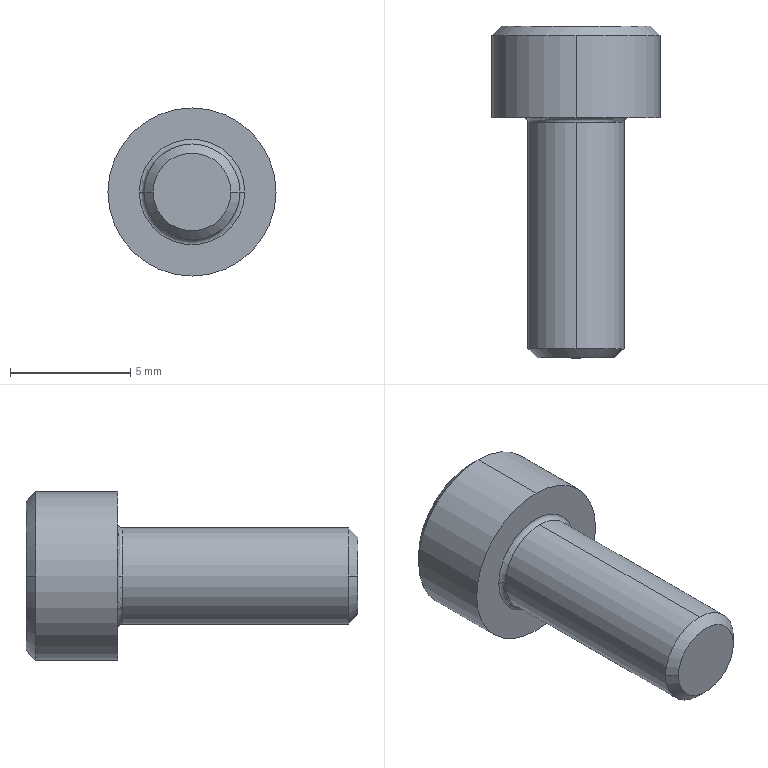Part | NX | 1 solid | 27 faces | box 7 x 13.82 x 7 mm | volume 252.618 mm3 | plane 15 | cone 6 | cylinder 4 | torus 2 | commonest cylinder face diameters 4 x2 7 x2
STEP:
#1=CARTESIAN_POINT('',(8.6,7.32,10.));
#2=VERTEX_POINT('',#1);
#3=CARTESIAN_POINT('',(2.4,7.32,10.));
#4=VERTEX_POINT('',#3);
#5=CARTESIAN_POINT('',(5.5,7.32,10.));
#6=DIRECTION('',(0.,1.,0.));
#7=DIRECTION('',(0.,0.,1.));
#8=AXIS2_PLACEMENT_3D('',#5,#6,#7);
#9=CIRCLE('',#8,3.1);
#10=EDGE_CURVE('',#2,#4,#9,.T.);
#11=ORIENTED_EDGE('',*,*,#10,.F.);
#12=CARTESIAN_POINT('',(9.,6.92,10.));
#13=VERTEX_POINT('',#12);
#14=CARTESIAN_POINT('',(8.8,7.12,10.));
#15=DIRECTION('',(0.7071,-0.7071,0.));
#16=VECTOR('',#15,1000.);
#17=LINE('',#14,#16);
#18=EDGE_CURVE('',#2,#13,#17,.T.);
#19=ORIENTED_EDGE('',*,*,#18,.T.);
#20=CARTESIAN_POINT('',(5.5,6.92,6.5));
#21=VERTEX_POINT('',#20);
#22=CARTESIAN_POINT('',(5.5,6.92,10.));
#23=DIRECTION('',(0.,1.,0.));
#24=DIRECTION('',(0.,0.,1.));
#25=AXIS2_PLACEMENT_3D('',#22,#23,#24);
#26=CIRCLE('',#25,3.5);
#27=EDGE_CURVE('',#13,#21,#26,.T.);
#28=ORIENTED_EDGE('',*,*,#27,.T.);
#29=CARTESIAN_POINT('',(2.,6.92,10.));
#30=VERTEX_POINT('',#29);
#31=CARTESIAN_POINT('',(5.5,6.92,10.));
#32=DIRECTION('',(0.,1.,0.));
#33=DIRECTION('',(0.,0.,1.));
#34=AXIS2_PLACEMENT_3D('',#31,#32,#33);
#35=CIRCLE('',#34,3.5);
#36=EDGE_CURVE('',#21,#30,#35,.T.);
#37=ORIENTED_EDGE('',*,*,#36,.T.);
#38=CARTESIAN_POINT('',(2.2,7.12,10.));
#39=DIRECTION('',(-0.7071,-0.7071,0.));
#40=VECTOR('',#39,1000.);
#41=LINE('',#38,#40);
#42=EDGE_CURVE('',#4,#30,#41,.T.);
#43=ORIENTED_EDGE('',*,*,#42,.F.);
#44=EDGE_LOOP('',(#11,#19,#28,#37,#43));
#45=FACE_BOUND('',#44,.T.);
#46=CARTESIAN_POINT('',(5.5,7.12,10.));
#47=DIRECTION('',(0.,-1.,0.));
#48=DIRECTION('',(-1.,0.,0.));
#49=AXIS2_PLACEMENT_3D('',#46,#47,#48);
#50=CONICAL_SURFACE('',#49,3.3,0.7854);
#51=ADVANCED_FACE('',(#45),#50,.T.);
#52=CARTESIAN_POINT('',(5.5,6.92,13.5));
#53=VERTEX_POINT('',#52);
#54=CARTESIAN_POINT('',(5.5,6.92,10.));
#55=DIRECTION('',(0.,1.,0.));
#56=DIRECTION('',(0.,0.,1.));
#57=AXIS2_PLACEMENT_3D('',#54,#55,#56);
#58=CIRCLE('',#57,3.5);
#59=EDGE_CURVE('',#30,#53,#58,.T.);
#60=ORIENTED_EDGE('',*,*,#59,.F.);
#61=ORIENTED_EDGE('',*,*,#36,.F.);
#62=CARTESIAN_POINT('',(5.5,3.5,6.5));
#63=VERTEX_POINT('',#62);
#64=CARTESIAN_POINT('',(5.5,5.21,6.5));
#65=DIRECTION('',(0.,-1.,0.));
#66=VECTOR('',#65,1000.);
#67=LINE('',#64,#66);
#68=EDGE_CURVE('',#21,#63,#67,.T.);
#69=ORIENTED_EDGE('',*,*,#68,.T.);
#70=CARTESIAN_POINT('',(5.5,3.5,13.5));
#71=VERTEX_POINT('',#70);
#72=CARTESIAN_POINT('',(5.5,3.5,10.));
#73=DIRECTION('',(0.,1.,0.));
#74=DIRECTION('',(0.,0.,1.));
#75=AXIS2_PLACEMENT_3D('',#72,#73,#74);
#76=CIRCLE('',#75,3.5);
#77=EDGE_CURVE('',#63,#71,#76,.T.);
#78=ORIENTED_EDGE('',*,*,#77,.T.);
#79=CARTESIAN_POINT('',(5.5,5.21,13.5));
#80=DIRECTION('',(0.,-1.,0.));
#81=VECTOR('',#80,1000.);
#82=LINE('',#79,#81);
#83=EDGE_CURVE('',#53,#71,#82,.T.);
#84=ORIENTED_EDGE('',*,*,#83,.F.);
#85=EDGE_LOOP('',(#60,#61,#69,#78,#84));
#86=FACE_BOUND('',#85,.T.);
#87=CARTESIAN_POINT('',(5.5,5.21,10.));
#88=DIRECTION('',(0.,-1.,0.));
#89=DIRECTION('',(0.,0.,1.));
#90=AXIS2_PLACEMENT_3D('',#87,#88,#89);
#91=CYLINDRICAL_SURFACE('',#90,3.5);
#92=ADVANCED_FACE('',(#86),#91,.T.);
#93=CARTESIAN_POINT('',(3.3,3.5,10.));
#94=VERTEX_POINT('',#93);
#95=CARTESIAN_POINT('',(7.7,3.5,10.));
#96=VERTEX_POINT('',#95);
#97=CARTESIAN_POINT('',(5.5,3.5,10.));
#98=DIRECTION('',(0.,1.,0.));
#99=DIRECTION('',(0.,0.,1.));
#100=AXIS2_PLACEMENT_3D('',#97,#98,#99);
#101=CIRCLE('',#100,2.2);
#102=EDGE_CURVE('',#94,#96,#101,.T.);
#103=ORIENTED_EDGE('',*,*,#102,.F.);
#104=CARTESIAN_POINT('',(3.5,3.3,10.));
#105=VERTEX_POINT('',#104);
#106=CARTESIAN_POINT('',(3.3,3.3,10.));
#107=DIRECTION('',(0.,0.,1.));
#108=DIRECTION('',(1.,0.,0.));
#109=AXIS2_PLACEMENT_3D('',#106,#107,#108);
#110=CIRCLE('',#109,0.2);
#111=EDGE_CURVE('',#94,#105,#110,.F.);
#112=ORIENTED_EDGE('',*,*,#111,.T.);
#113=CARTESIAN_POINT('',(5.5,3.3,12.));
#114=VERTEX_POINT('',#113);
#115=CARTESIAN_POINT('',(5.5,3.3,10.));
#116=DIRECTION('',(0.,1.,0.));
#117=DIRECTION('',(1.,0.,0.));
#118=AXIS2_PLACEMENT_3D('',#115,#116,#117);
#119=CIRCLE('',#118,2.);
#120=EDGE_CURVE('',#105,#114,#119,.T.);
#121=ORIENTED_EDGE('',*,*,#120,.T.);
#122=CARTESIAN_POINT('',(7.5,3.3,10.));
#123=VERTEX_POINT('',#122);
#124=CARTESIAN_POINT('',(5.5,3.3,10.));
#125=DIRECTION('',(0.,1.,0.));
#126=DIRECTION('',(1.,0.,0.));
#127=AXIS2_PLACEMENT_3D('',#124,#125,#126);
#128=CIRCLE('',#127,2.);
#129=EDGE_CURVE('',#114,#123,#128,.T.);
#130=ORIENTED_EDGE('',*,*,#129,.T.);
#131=CARTESIAN_POINT('',(7.7,3.3,10.));
#132=DIRECTION('',(0.,0.,-1.));
#133=DIRECTION('',(-1.,0.,0.));
#134=AXIS2_PLACEMENT_3D('',#131,#132,#133);
#135=CIRCLE('',#134,0.2);
#136=EDGE_CURVE('',#96,#123,#135,.F.);
#137=ORIENTED_EDGE('',*,*,#136,.F.);
#138=EDGE_LOOP('',(#103,#112,#121,#130,#137));
#139=FACE_BOUND('',#138,.T.);
#140=CARTESIAN_POINT('',(5.5,3.3,10.));
#141=DIRECTION('',(0.,1.,0.));
#142=DIRECTION('',(1.,0.,0.));
#143=AXIS2_PLACEMENT_3D('',#140,#141,#142);
#144=TOROIDAL_SURFACE('',#143,2.2,0.2);
#145=ADVANCED_FACE('',(#139),#144,.F.);
#146=CARTESIAN_POINT('',(5.5,-6.121,8.));
#147=VERTEX_POINT('',#146);
#148=CARTESIAN_POINT('',(3.5,-6.121,10.));
#149=VERTEX_POINT('',#148);
#150=CARTESIAN_POINT('',(5.5,-6.121,10.));
#151=DIRECTION('',(0.,1.,0.));
#152=DIRECTION('',(0.,0.,1.));
#153=AXIS2_PLACEMENT_3D('',#150,#151,#152);
#154=CIRCLE('',#153,2.);
#155=EDGE_CURVE('',#147,#149,#154,.T.);
#156=ORIENTED_EDGE('',*,*,#155,.T.);
#157=CARTESIAN_POINT('',(5.5,-6.121,12.));
#158=VERTEX_POINT('',#157);
#159=CARTESIAN_POINT('',(5.5,-6.121,10.));
#160=DIRECTION('',(0.,1.,0.));
#161=DIRECTION('',(0.,0.,1.));
#162=AXIS2_PLACEMENT_3D('',#159,#160,#161);
#163=CIRCLE('',#162,2.);
#164=EDGE_CURVE('',#149,#158,#163,.T.);
#165=ORIENTED_EDGE('',*,*,#164,.T.);
#166=CARTESIAN_POINT('',(5.5,-1.411,12.));
#167=DIRECTION('',(0.,-1.,0.));
#168=VECTOR('',#167,1000.);
#169=LINE('',#166,#168);
#170=EDGE_CURVE('',#114,#158,#169,.T.);
#171=ORIENTED_EDGE('',*,*,#170,.F.);
#172=ORIENTED_EDGE('',*,*,#120,.F.);
#173=CARTESIAN_POINT('',(5.5,3.3,8.));
#174=VERTEX_POINT('',#173);
#175=CARTESIAN_POINT('',(5.5,3.3,10.));
#176=DIRECTION('',(0.,1.,0.));
#177=DIRECTION('',(1.,0.,0.));
#178=AXIS2_PLACEMENT_3D('',#175,#176,#177);
#179=CIRCLE('',#178,2.);
#180=EDGE_CURVE('',#174,#105,#179,.T.);
#181=ORIENTED_EDGE('',*,*,#180,.F.);
#182=CARTESIAN_POINT('',(5.5,-1.411,8.));
#183=DIRECTION('',(0.,-1.,0.));
#184=VECTOR('',#183,1000.);
#185=LINE('',#182,#184);
#186=EDGE_CURVE('',#174,#147,#185,.T.);
#187=ORIENTED_EDGE('',*,*,#186,.T.);
#188=EDGE_LOOP('',(#156,#165,#171,#172,#181,#187));
#189=FACE_BOUND('',#188,.T.);
#190=CARTESIAN_POINT('',(5.5,-1.411,10.));
#191=DIRECTION('',(0.,-1.,0.));
#192=DIRECTION('',(0.,0.,1.));
#193=AXIS2_PLACEMENT_3D('',#190,#191,#192);
#194=CYLINDRICAL_SURFACE('',#193,2.);
#195=ADVANCED_FACE('',(#189),#194,.T.);
#196=ORIENTED_EDGE('',*,*,#155,.F.);
#197=CARTESIAN_POINT('',(7.5,-6.121,10.));
#198=VERTEX_POINT('',#197);
#199=CARTESIAN_POINT('',(5.5,-6.121,10.));
#200=DIRECTION('',(0.,1.,0.));
#201=DIRECTION('',(0.,0.,1.));
#202=AXIS2_PLACEMENT_3D('',#199,#200,#201);
#203=CIRCLE('',#202,2.);
#204=EDGE_CURVE('',#198,#147,#203,.T.);
#205=ORIENTED_EDGE('',*,*,#204,.F.);
#206=CARTESIAN_POINT('',(7.121,-6.5,10.));
#207=VERTEX_POINT('',#206);
#208=CARTESIAN_POINT('',(7.311,-6.311,10.));
#209=DIRECTION('',(0.7071,0.7071,0.));
#210=VECTOR('',#209,1000.);
#211=LINE('',#208,#210);
#212=EDGE_CURVE('',#207,#198,#211,.T.);
#213=ORIENTED_EDGE('',*,*,#212,.F.);
#214=CARTESIAN_POINT('',(3.879,-6.5,10.));
#215=VERTEX_POINT('',#214);
#216=CARTESIAN_POINT('',(5.5,-6.5,10.));
#217=DIRECTION('',(0.,1.,0.));
#218=DIRECTION('',(0.,0.,1.));
#219=AXIS2_PLACEMENT_3D('',#216,#217,#218);
#220=CIRCLE('',#219,1.621);
#221=EDGE_CURVE('',#207,#215,#220,.T.);
#222=ORIENTED_EDGE('',*,*,#221,.T.);
#223=CARTESIAN_POINT('',(3.689,-6.311,10.));
#224=DIRECTION('',(-0.7071,0.7071,0.));
#225=VECTOR('',#224,1000.);
#226=LINE('',#223,#225);
#227=EDGE_CURVE('',#215,#149,#226,.T.);
#228=ORIENTED_EDGE('',*,*,#227,.T.);
#229=EDGE_LOOP('',(#196,#205,#213,#222,#228));
#230=FACE_BOUND('',#229,.T.);
#231=CARTESIAN_POINT('',(5.5,-6.311,10.));
#232=DIRECTION('',(0.,1.,0.));
#233=DIRECTION('',(1.,0.,0.));
#234=AXIS2_PLACEMENT_3D('',#231,#232,#233);
#235=CONICAL_SURFACE('',#234,1.81,0.7854);
#236=ADVANCED_FACE('',(#230),#235,.T.);
#237=CARTESIAN_POINT('',(4.,5.32,10.));
#238=VERTEX_POINT('',#237);
#239=CARTESIAN_POINT('',(5.5,4.454,10.));
#240=VERTEX_POINT('',#239);
#241=CARTESIAN_POINT('',(4.75,4.887,10.));
#242=DIRECTION('',(-0.866,0.5,0.));
#243=VECTOR('',#242,1000.);
#244=LINE('',#241,#243);
#245=EDGE_CURVE('',#238,#240,#244,.F.);
#246=ORIENTED_EDGE('',*,*,#245,.F.);
#247=CARTESIAN_POINT('',(4.75,5.32,11.299));
#248=VERTEX_POINT('',#247);
#249=CARTESIAN_POINT('',(5.5,5.32,10.));
#250=DIRECTION('',(0.,-1.,0.));
#251=DIRECTION('',(0.,0.,1.));
#252=AXIS2_PLACEMENT_3D('',#249,#250,#251);
#253=CIRCLE('',#252,1.5);
#254=EDGE_CURVE('',#248,#238,#253,.T.);
#255=ORIENTED_EDGE('',*,*,#254,.F.);
#256=CARTESIAN_POINT('',(6.25,5.32,11.299));
#257=VERTEX_POINT('',#256);
#258=CARTESIAN_POINT('',(5.5,5.32,10.));
#259=DIRECTION('',(0.,-1.,0.));
#260=DIRECTION('',(0.,0.,1.));
#261=AXIS2_PLACEMENT_3D('',#258,#259,#260);
#262=CIRCLE('',#261,1.5);
#263=EDGE_CURVE('',#257,#248,#262,.T.);
#264=ORIENTED_EDGE('',*,*,#263,.F.);
#265=CARTESIAN_POINT('',(7.,5.32,10.));
#266=VERTEX_POINT('',#265);
#267=CARTESIAN_POINT('',(5.5,5.32,10.));
#268=DIRECTION('',(0.,-1.,0.));
#269=DIRECTION('',(0.,0.,1.));
#270=AXIS2_PLACEMENT_3D('',#267,#268,#269);
#271=CIRCLE('',#270,1.5);
#272=EDGE_CURVE('',#266,#257,#271,.T.);
#273=ORIENTED_EDGE('',*,*,#272,.F.);
#274=CARTESIAN_POINT('',(6.25,4.887,10.));
#275=DIRECTION('',(0.866,0.5,0.));
#276=VECTOR('',#275,1000.);
#277=LINE('',#274,#276);
#278=EDGE_CURVE('',#266,#240,#277,.F.);
#279=ORIENTED_EDGE('',*,*,#278,.T.);
#280=EDGE_LOOP('',(#246,#255,#264,#273,#279));
#281=FACE_BOUND('',#280,.T.);
#282=CARTESIAN_POINT('',(5.5,4.887,10.));
#283=DIRECTION('',(0.,1.,0.));
#284=DIRECTION('',(1.,0.,0.));
#285=AXIS2_PLACEMENT_3D('',#282,#283,#284);
#286=CONICAL_SURFACE('',#285,0.75,1.047);
#287=ADVANCED_FACE('',(#281),#286,.F.);
#288=ORIENTED_EDGE('',*,*,#10,.T.);
#289=CARTESIAN_POINT('',(5.5,7.32,10.));
#290=DIRECTION('',(0.,1.,0.));
#291=DIRECTION('',(0.,0.,1.));
#292=AXIS2_PLACEMENT_3D('',#289,#290,#291);
#293=CIRCLE('',#292,3.1);
#294=EDGE_CURVE('',#4,#2,#293,.T.);
#295=ORIENTED_EDGE('',*,*,#294,.T.);
#296=EDGE_LOOP('',(#288,#295));
#297=FACE_BOUND('',#296,.T.);
#298=CARTESIAN_POINT('',(5.5,7.32,11.732));
#299=VERTEX_POINT('',#298);
#300=CARTESIAN_POINT('',(4.,7.32,10.866));
#301=VERTEX_POINT('',#300);
#302=CARTESIAN_POINT('',(4.711,7.32,11.276));
#303=DIRECTION('',(-0.866,0.,-0.5));
#304=VECTOR('',#303,1000.);
#305=LINE('',#302,#304);
#306=EDGE_CURVE('',#299,#301,#305,.T.);
#307=ORIENTED_EDGE('',*,*,#306,.T.);
#308=CARTESIAN_POINT('',(4.,7.32,9.134));
#309=VERTEX_POINT('',#308);
#310=CARTESIAN_POINT('',(4.,7.32,10.342));
#311=DIRECTION('',(0.,0.,-1.));
#312=VECTOR('',#311,1000.);
#313=LINE('',#310,#312);
#314=EDGE_CURVE('',#301,#309,#313,.T.);
#315=ORIENTED_EDGE('',*,*,#314,.T.);
#316=CARTESIAN_POINT('',(5.5,7.32,8.268));
#317=VERTEX_POINT('',#316);
#318=CARTESIAN_POINT('',(4.789,7.32,8.678));
#319=DIRECTION('',(0.866,0.,-0.5));
#320=VECTOR('',#319,1000.);
#321=LINE('',#318,#320);
#322=EDGE_CURVE('',#309,#317,#321,.T.);
#323=ORIENTED_EDGE('',*,*,#322,.T.);
#324=CARTESIAN_POINT('',(7.,7.32,9.134));
#325=VERTEX_POINT('',#324);
#326=CARTESIAN_POINT('',(6.961,7.32,9.111));
#327=DIRECTION('',(0.866,0.,0.5));
#328=VECTOR('',#327,1000.);
#329=LINE('',#326,#328);
#330=EDGE_CURVE('',#317,#325,#329,.T.);
#331=ORIENTED_EDGE('',*,*,#330,.T.);
#332=CARTESIAN_POINT('',(7.,7.32,10.866));
#333=VERTEX_POINT('',#332);
#334=CARTESIAN_POINT('',(7.,7.32,11.208));
#335=DIRECTION('',(0.,0.,1.));
#336=VECTOR('',#335,1000.);
#337=LINE('',#334,#336);
#338=EDGE_CURVE('',#325,#333,#337,.T.);
#339=ORIENTED_EDGE('',*,*,#338,.T.);
#340=CARTESIAN_POINT('',(5.539,7.32,11.709));
#341=DIRECTION('',(-0.866,0.,0.5));
#342=VECTOR('',#341,1000.);
#343=LINE('',#340,#342);
#344=EDGE_CURVE('',#333,#299,#343,.T.);
#345=ORIENTED_EDGE('',*,*,#344,.T.);
#346=EDGE_LOOP('',(#307,#315,#323,#331,#339,#345));
#347=FACE_BOUND('',#346,.T.);
#348=CARTESIAN_POINT('',(5.5,7.32,11.55));
#349=DIRECTION('',(0.,1.,0.));
#350=DIRECTION('',(1.,0.,0.));
#351=AXIS2_PLACEMENT_3D('',#348,#349,#350);
#352=PLANE('',#351);
#353=ADVANCED_FACE('',(#297,#347),#352,.T.);
#354=CARTESIAN_POINT('',(6.25,5.32,8.701));
#355=VERTEX_POINT('',#354);
#356=CARTESIAN_POINT('',(5.5,5.32,10.));
#357=DIRECTION('',(0.,-1.,0.));
#358=DIRECTION('',(0.,0.,1.));
#359=AXIS2_PLACEMENT_3D('',#356,#357,#358);
#360=CIRCLE('',#359,1.5);
#361=EDGE_CURVE('',#355,#266,#360,.T.);
#362=ORIENTED_EDGE('',*,*,#361,.T.);
#363=CARTESIAN_POINT('',(7.,5.32,9.134));
#364=VERTEX_POINT('',#363);
#365=CARTESIAN_POINT('',(7.,5.32,9.134));
#366=DIRECTION('',(0.,0.,-1.));
#367=VECTOR('',#366,1000.);
#368=LINE('',#365,#367);
#369=EDGE_CURVE('',#266,#364,#368,.T.);
#370=ORIENTED_EDGE('',*,*,#369,.T.);
#371=CARTESIAN_POINT('',(5.5,5.32,8.268));
#372=DIRECTION('',(-0.866,0.,-0.5));
#373=VECTOR('',#372,1000.);
#374=LINE('',#371,#373);
#375=EDGE_CURVE('',#364,#355,#374,.T.);
#376=ORIENTED_EDGE('',*,*,#375,.T.);
#377=EDGE_LOOP('',(#362,#370,#376));
#378=FACE_BOUND('',#377,.T.);
#379=CARTESIAN_POINT('',(5.5,5.32,10.));
#380=DIRECTION('',(0.,-1.,0.));
#381=DIRECTION('',(0.,0.,-1.));
#382=AXIS2_PLACEMENT_3D('',#379,#380,#381);
#383=PLANE('',#382);
#384=ADVANCED_FACE('',(#378),#383,.F.);
#385=ORIENTED_EDGE('',*,*,#272,.T.);
#386=CARTESIAN_POINT('',(7.,5.32,10.866));
#387=VERTEX_POINT('',#386);
#388=CARTESIAN_POINT('',(7.,5.32,10.866));
#389=DIRECTION('',(0.866,0.,-0.5));
#390=VECTOR('',#389,1000.);
#391=LINE('',#388,#390);
#392=EDGE_CURVE('',#257,#387,#391,.T.);
#393=ORIENTED_EDGE('',*,*,#392,.T.);
#394=CARTESIAN_POINT('',(7.,5.32,9.134));
#395=DIRECTION('',(0.,0.,-1.));
#396=VECTOR('',#395,1000.);
#397=LINE('',#394,#396);
#398=EDGE_CURVE('',#387,#266,#397,.T.);
#399=ORIENTED_EDGE('',*,*,#398,.T.);
#400=EDGE_LOOP('',(#385,#393,#399));
#401=FACE_BOUND('',#400,.T.);
#402=CARTESIAN_POINT('',(5.5,5.32,10.));
#403=DIRECTION('',(0.,-1.,0.));
#404=DIRECTION('',(0.,0.,-1.));
#405=AXIS2_PLACEMENT_3D('',#402,#403,#404);
#406=PLANE('',#405);
#407=ADVANCED_FACE('',(#401),#406,.F.);
#408=ORIENTED_EDGE('',*,*,#263,.T.);
#409=CARTESIAN_POINT('',(5.5,5.32,11.732));
#410=VERTEX_POINT('',#409);
#411=CARTESIAN_POINT('',(5.5,5.32,11.732));
#412=DIRECTION('',(0.866,0.,0.5));
#413=VECTOR('',#412,1000.);
#414=LINE('',#411,#413);
#415=EDGE_CURVE('',#248,#410,#414,.T.);
#416=ORIENTED_EDGE('',*,*,#415,.T.);
#417=CARTESIAN_POINT('',(7.,5.32,10.866));
#418=DIRECTION('',(0.866,0.,-0.5));
#419=VECTOR('',#418,1000.);
#420=LINE('',#417,#419);
#421=EDGE_CURVE('',#410,#257,#420,.T.);
#422=ORIENTED_EDGE('',*,*,#421,.T.);
#423=EDGE_LOOP('',(#408,#416,#422));
#424=FACE_BOUND('',#423,.T.);
#425=CARTESIAN_POINT('',(5.5,5.32,10.));
#426=DIRECTION('',(0.,-1.,0.));
#427=DIRECTION('',(0.,0.,-1.));
#428=AXIS2_PLACEMENT_3D('',#425,#426,#427);
#429=PLANE('',#428);
#430=ADVANCED_FACE('',(#424),#429,.F.);
#431=ORIENTED_EDGE('',*,*,#254,.T.);
#432=CARTESIAN_POINT('',(4.,5.32,10.866));
#433=VERTEX_POINT('',#432);
#434=CARTESIAN_POINT('',(4.,5.32,10.866));
#435=DIRECTION('',(0.,0.,1.));
#436=VECTOR('',#435,1000.);
#437=LINE('',#434,#436);
#438=EDGE_CURVE('',#238,#433,#437,.T.);
#439=ORIENTED_EDGE('',*,*,#438,.T.);
#440=CARTESIAN_POINT('',(5.5,5.32,11.732));
#441=DIRECTION('',(0.866,0.,0.5));
#442=VECTOR('',#441,1000.);
#443=LINE('',#440,#442);
#444=EDGE_CURVE('',#433,#248,#443,.T.);
#445=ORIENTED_EDGE('',*,*,#444,.T.);
#446=EDGE_LOOP('',(#431,#439,#445));
#447=FACE_BOUND('',#446,.T.);
#448=CARTESIAN_POINT('',(5.5,5.32,10.));
#449=DIRECTION('',(0.,-1.,0.));
#450=DIRECTION('',(0.,0.,-1.));
#451=AXIS2_PLACEMENT_3D('',#448,#449,#450);
#452=PLANE('',#451);
#453=ADVANCED_FACE('',(#447),#452,.F.);
#454=CARTESIAN_POINT('',(4.75,5.32,8.701));
#455=VERTEX_POINT('',#454);
#456=CARTESIAN_POINT('',(5.5,5.32,10.));
#457=DIRECTION('',(0.,-1.,0.));
#458=DIRECTION('',(0.,0.,1.));
#459=AXIS2_PLACEMENT_3D('',#456,#457,#458);
#460=CIRCLE('',#459,1.5);
#461=EDGE_CURVE('',#238,#455,#460,.T.);
#462=ORIENTED_EDGE('',*,*,#461,.T.);
#463=CARTESIAN_POINT('',(4.,5.32,9.134));
#464=VERTEX_POINT('',#463);
#465=CARTESIAN_POINT('',(4.,5.32,9.134));
#466=DIRECTION('',(-0.866,0.,0.5));
#467=VECTOR('',#466,1000.);
#468=LINE('',#465,#467);
#469=EDGE_CURVE('',#455,#464,#468,.T.);
#470=ORIENTED_EDGE('',*,*,#469,.T.);
#471=CARTESIAN_POINT('',(4.,5.32,10.866));
#472=DIRECTION('',(0.,0.,1.));
#473=VECTOR('',#472,1000.);
#474=LINE('',#471,#473);
#475=EDGE_CURVE('',#464,#238,#474,.T.);
#476=ORIENTED_EDGE('',*,*,#475,.T.);
#477=EDGE_LOOP('',(#462,#470,#476));
#478=FACE_BOUND('',#477,.T.);
#479=CARTESIAN_POINT('',(5.5,5.32,10.));
#480=DIRECTION('',(0.,-1.,0.));
#481=DIRECTION('',(0.,0.,-1.));
#482=AXIS2_PLACEMENT_3D('',#479,#480,#481);
#483=PLANE('',#482);
#484=ADVANCED_FACE('',(#478),#483,.F.);
#485=CARTESIAN_POINT('',(5.5,5.32,10.));
#486=DIRECTION('',(0.,-1.,0.));
#487=DIRECTION('',(0.,0.,1.));
#488=AXIS2_PLACEMENT_3D('',#485,#486,#487);
#489=CIRCLE('',#488,1.5);
#490=EDGE_CURVE('',#455,#355,#489,.T.);
#491=ORIENTED_EDGE('',*,*,#490,.T.);
#492=CARTESIAN_POINT('',(5.5,5.32,8.268));
#493=VERTEX_POINT('',#492);
#494=CARTESIAN_POINT('',(5.5,5.32,8.268));
#495=DIRECTION('',(-0.866,0.,-0.5));
#496=VECTOR('',#495,1000.);
#497=LINE('',#494,#496);
#498=EDGE_CURVE('',#355,#493,#497,.T.);
#499=ORIENTED_EDGE('',*,*,#498,.T.);
#500=CARTESIAN_POINT('',(4.,5.32,9.134));
#501=DIRECTION('',(-0.866,0.,0.5));
#502=VECTOR('',#501,1000.);
#503=LINE('',#500,#502);
#504=EDGE_CURVE('',#493,#455,#503,.T.);
#505=ORIENTED_EDGE('',*,*,#504,.T.);
#506=EDGE_LOOP('',(#491,#499,#505));
#507=FACE_BOUND('',#506,.T.);
#508=CARTESIAN_POINT('',(5.5,5.32,10.));
#509=DIRECTION('',(0.,-1.,0.));
#510=DIRECTION('',(0.,0.,-1.));
#511=AXIS2_PLACEMENT_3D('',#508,#509,#510);
#512=PLANE('',#511);
#513=ADVANCED_FACE('',(#507),#512,.F.);
#514=ORIENTED_EDGE('',*,*,#444,.F.);
#515=CARTESIAN_POINT('',(4.,7.32,10.866));
#516=DIRECTION('',(0.,-1.,0.));
#517=VECTOR('',#516,1000.);
#518=LINE('',#515,#517);
#519=EDGE_CURVE('',#301,#433,#518,.T.);
#520=ORIENTED_EDGE('',*,*,#519,.F.);
#521=ORIENTED_EDGE('',*,*,#306,.F.);
#522=CARTESIAN_POINT('',(5.5,7.32,11.732));
#523=DIRECTION('',(0.,-1.,0.));
#524=VECTOR('',#523,1000.);
#525=LINE('',#522,#524);
#526=EDGE_CURVE('',#299,#410,#525,.T.);
#527=ORIENTED_EDGE('',*,*,#526,.T.);
#528=ORIENTED_EDGE('',*,*,#415,.F.);
#529=EDGE_LOOP('',(#514,#520,#521,#527,#528));
#530=FACE_BOUND('',#529,.T.);
#531=CARTESIAN_POINT('',(4.,7.32,10.866));
#532=DIRECTION('',(-0.5,0.,0.866));
#533=DIRECTION('',(0.,1.,0.));
#534=AXIS2_PLACEMENT_3D('',#531,#532,#533);
#535=PLANE('',#534);
#536=ADVANCED_FACE('',(#530),#535,.F.);
#537=ORIENTED_EDGE('',*,*,#421,.F.);
#538=ORIENTED_EDGE('',*,*,#526,.F.);
#539=ORIENTED_EDGE('',*,*,#344,.F.);
#540=CARTESIAN_POINT('',(7.,7.32,10.866));
#541=DIRECTION('',(0.,-1.,0.));
#542=VECTOR('',#541,1000.);
#543=LINE('',#540,#542);
#544=EDGE_CURVE('',#333,#387,#543,.T.);
#545=ORIENTED_EDGE('',*,*,#544,.T.);
#546=ORIENTED_EDGE('',*,*,#392,.F.);
#547=EDGE_LOOP('',(#537,#538,#539,#545,#546));
#548=FACE_BOUND('',#547,.T.);
#549=CARTESIAN_POINT('',(5.5,7.32,11.732));
#550=DIRECTION('',(0.5,0.,0.866));
#551=DIRECTION('',(0.,-1.,0.));
#552=AXIS2_PLACEMENT_3D('',#549,#550,#551);
#553=PLANE('',#552);
#554=ADVANCED_FACE('',(#548),#553,.F.);
#555=ORIENTED_EDGE('',*,*,#398,.F.);
#556=ORIENTED_EDGE('',*,*,#544,.F.);
#557=ORIENTED_EDGE('',*,*,#338,.F.);
#558=CARTESIAN_POINT('',(7.,7.32,9.134));
#559=DIRECTION('',(0.,-1.,0.));
#560=VECTOR('',#559,1000.);
#561=LINE('',#558,#560);
#562=EDGE_CURVE('',#325,#364,#561,.T.);
#563=ORIENTED_EDGE('',*,*,#562,.T.);
#564=ORIENTED_EDGE('',*,*,#369,.F.);
#565=EDGE_LOOP('',(#555,#556,#557,#563,#564));
#566=FACE_BOUND('',#565,.T.);
#567=CARTESIAN_POINT('',(7.,7.32,10.866));
#568=DIRECTION('',(1.,0.,0.));
#569=DIRECTION('',(0.,1.,0.));
#570=AXIS2_PLACEMENT_3D('',#567,#568,#569);
#571=PLANE('',#570);
#572=ADVANCED_FACE('',(#566),#571,.F.);
#573=ORIENTED_EDGE('',*,*,#375,.F.);
#574=ORIENTED_EDGE('',*,*,#562,.F.);
#575=ORIENTED_EDGE('',*,*,#330,.F.);
#576=CARTESIAN_POINT('',(5.5,7.32,8.268));
#577=DIRECTION('',(0.,-1.,0.));
#578=VECTOR('',#577,1000.);
#579=LINE('',#576,#578);
#580=EDGE_CURVE('',#317,#493,#579,.T.);
#581=ORIENTED_EDGE('',*,*,#580,.T.);
#582=ORIENTED_EDGE('',*,*,#498,.F.);
#583=EDGE_LOOP('',(#573,#574,#575,#581,#582));
#584=FACE_BOUND('',#583,.T.);
#585=CARTESIAN_POINT('',(7.,7.32,9.134));
#586=DIRECTION('',(0.5,0.,-0.866));
#587=DIRECTION('',(0.,-1.,0.));
#588=AXIS2_PLACEMENT_3D('',#585,#586,#587);
#589=PLANE('',#588);
#590=ADVANCED_FACE('',(#584),#589,.F.);
#591=ORIENTED_EDGE('',*,*,#504,.F.);
#592=ORIENTED_EDGE('',*,*,#580,.F.);
#593=ORIENTED_EDGE('',*,*,#322,.F.);
#594=CARTESIAN_POINT('',(4.,7.32,9.134));
#595=DIRECTION('',(0.,-1.,0.));
#596=VECTOR('',#595,1000.);
#597=LINE('',#594,#596);
#598=EDGE_CURVE('',#309,#464,#597,.T.);
#599=ORIENTED_EDGE('',*,*,#598,.T.);
#600=ORIENTED_EDGE('',*,*,#469,.F.);
#601=EDGE_LOOP('',(#591,#592,#593,#599,#600));
#602=FACE_BOUND('',#601,.T.);
#603=CARTESIAN_POINT('',(5.5,7.32,8.268));
#604=DIRECTION('',(-0.5,0.,-0.866));
#605=DIRECTION('',(-0.866,0.,0.5));
#606=AXIS2_PLACEMENT_3D('',#603,#604,#605);
#607=PLANE('',#606);
#608=ADVANCED_FACE('',(#602),#607,.F.);
#609=ORIENTED_EDGE('',*,*,#475,.F.);
#610=ORIENTED_EDGE('',*,*,#598,.F.);
#611=ORIENTED_EDGE('',*,*,#314,.F.);
#612=ORIENTED_EDGE('',*,*,#519,.T.);
#613=ORIENTED_EDGE('',*,*,#438,.F.);
#614=EDGE_LOOP('',(#609,#610,#611,#612,#613));
#615=FACE_BOUND('',#614,.T.);
#616=CARTESIAN_POINT('',(4.,7.32,9.134));
#617=DIRECTION('',(-1.,0.,0.));
#618=DIRECTION('',(0.,0.,1.));
#619=AXIS2_PLACEMENT_3D('',#616,#617,#618);
#620=PLANE('',#619);
#621=ADVANCED_FACE('',(#615),#620,.F.);
#622=ORIENTED_EDGE('',*,*,#221,.F.);
#623=CARTESIAN_POINT('',(5.5,-6.5,10.));
#624=DIRECTION('',(0.,1.,0.));
#625=DIRECTION('',(0.,0.,1.));
#626=AXIS2_PLACEMENT_3D('',#623,#624,#625);
#627=CIRCLE('',#626,1.621);
#628=EDGE_CURVE('',#215,#207,#627,.T.);
#629=ORIENTED_EDGE('',*,*,#628,.F.);
#630=EDGE_LOOP('',(#622,#629));
#631=FACE_BOUND('',#630,.T.);
#632=CARTESIAN_POINT('',(5.5,-6.5,10.81));
#633=DIRECTION('',(0.,-1.,0.));
#634=DIRECTION('',(0.,0.,-1.));
#635=AXIS2_PLACEMENT_3D('',#632,#633,#634);
#636=PLANE('',#635);
#637=ADVANCED_FACE('',(#631),#636,.T.);
#638=ORIENTED_EDGE('',*,*,#77,.F.);
#639=CARTESIAN_POINT('',(5.5,3.5,10.));
#640=DIRECTION('',(0.,1.,0.));
#641=DIRECTION('',(0.,0.,1.));
#642=AXIS2_PLACEMENT_3D('',#639,#640,#641);
#643=CIRCLE('',#642,3.5);
#644=EDGE_CURVE('',#71,#63,#643,.T.);
#645=ORIENTED_EDGE('',*,*,#644,.F.);
#646=EDGE_LOOP('',(#638,#645));
#647=FACE_BOUND('',#646,.T.);
#648=ORIENTED_EDGE('',*,*,#102,.T.);
#649=CARTESIAN_POINT('',(5.5,3.5,10.));
#650=DIRECTION('',(0.,1.,0.));
#651=DIRECTION('',(0.,0.,1.));
#652=AXIS2_PLACEMENT_3D('',#649,#650,#651);
#653=CIRCLE('',#652,2.2);
#654=EDGE_CURVE('',#96,#94,#653,.T.);
#655=ORIENTED_EDGE('',*,*,#654,.T.);
#656=EDGE_LOOP('',(#648,#655));
#657=FACE_BOUND('',#656,.T.);
#658=CARTESIAN_POINT('',(5.5,3.5,12.85));
#659=DIRECTION('',(0.,-1.,0.));
#660=DIRECTION('',(0.,0.,-1.));
#661=AXIS2_PLACEMENT_3D('',#658,#659,#660);
#662=PLANE('',#661);
#663=ADVANCED_FACE('',(#647,#657),#662,.T.);
#664=ORIENTED_EDGE('',*,*,#212,.T.);
#665=CARTESIAN_POINT('',(5.5,-6.121,10.));
#666=DIRECTION('',(0.,1.,0.));
#667=DIRECTION('',(0.,0.,1.));
#668=AXIS2_PLACEMENT_3D('',#665,#666,#667);
#669=CIRCLE('',#668,2.);
#670=EDGE_CURVE('',#158,#198,#669,.T.);
#671=ORIENTED_EDGE('',*,*,#670,.F.);
#672=ORIENTED_EDGE('',*,*,#164,.F.);
#673=ORIENTED_EDGE('',*,*,#227,.F.);
#674=ORIENTED_EDGE('',*,*,#628,.T.);
#675=EDGE_LOOP('',(#664,#671,#672,#673,#674));
#676=FACE_BOUND('',#675,.T.);
#677=CARTESIAN_POINT('',(5.5,-6.311,10.));
#678=DIRECTION('',(0.,1.,0.));
#679=DIRECTION('',(1.,0.,0.));
#680=AXIS2_PLACEMENT_3D('',#677,#678,#679);
#681=CONICAL_SURFACE('',#680,1.81,0.7854);
#682=ADVANCED_FACE('',(#676),#681,.T.);
#683=ORIENTED_EDGE('',*,*,#170,.T.);
#684=ORIENTED_EDGE('',*,*,#670,.T.);
#685=ORIENTED_EDGE('',*,*,#204,.T.);
#686=ORIENTED_EDGE('',*,*,#186,.F.);
#687=CARTESIAN_POINT('',(5.5,3.3,10.));
#688=DIRECTION('',(0.,1.,0.));
#689=DIRECTION('',(1.,0.,0.));
#690=AXIS2_PLACEMENT_3D('',#687,#688,#689);
#691=CIRCLE('',#690,2.);
#692=EDGE_CURVE('',#123,#174,#691,.T.);
#693=ORIENTED_EDGE('',*,*,#692,.F.);
#694=ORIENTED_EDGE('',*,*,#129,.F.);
#695=EDGE_LOOP('',(#683,#684,#685,#686,#693,#694));
#696=FACE_BOUND('',#695,.T.);
#697=CARTESIAN_POINT('',(5.5,-1.411,10.));
#698=DIRECTION('',(0.,-1.,0.));
#699=DIRECTION('',(0.,0.,1.));
#700=AXIS2_PLACEMENT_3D('',#697,#698,#699);
#701=CYLINDRICAL_SURFACE('',#700,2.);
#702=ADVANCED_FACE('',(#696),#701,.T.);
#703=ORIENTED_EDGE('',*,*,#83,.T.);
#704=ORIENTED_EDGE('',*,*,#644,.T.);
#705=ORIENTED_EDGE('',*,*,#68,.F.);
#706=ORIENTED_EDGE('',*,*,#27,.F.);
#707=CARTESIAN_POINT('',(5.5,6.92,10.));
#708=DIRECTION('',(0.,1.,0.));
#709=DIRECTION('',(0.,0.,1.));
#710=AXIS2_PLACEMENT_3D('',#707,#708,#709);
#711=CIRCLE('',#710,3.5);
#712=EDGE_CURVE('',#53,#13,#711,.T.);
#713=ORIENTED_EDGE('',*,*,#712,.F.);
#714=EDGE_LOOP('',(#703,#704,#705,#706,#713));
#715=FACE_BOUND('',#714,.T.);
#716=CARTESIAN_POINT('',(5.5,5.21,10.));
#717=DIRECTION('',(0.,-1.,0.));
#718=DIRECTION('',(0.,0.,1.));
#719=AXIS2_PLACEMENT_3D('',#716,#717,#718);
#720=CYLINDRICAL_SURFACE('',#719,3.5);
#721=ADVANCED_FACE('',(#715),#720,.T.);
#722=ORIENTED_EDGE('',*,*,#59,.T.);
#723=ORIENTED_EDGE('',*,*,#712,.T.);
#724=ORIENTED_EDGE('',*,*,#18,.F.);
#725=ORIENTED_EDGE('',*,*,#294,.F.);
#726=ORIENTED_EDGE('',*,*,#42,.T.);
#727=EDGE_LOOP('',(#722,#723,#724,#725,#726));
#728=FACE_BOUND('',#727,.T.);
#729=CARTESIAN_POINT('',(5.5,7.12,10.));
#730=DIRECTION('',(0.,-1.,0.));
#731=DIRECTION('',(-1.,0.,0.));
#732=AXIS2_PLACEMENT_3D('',#729,#730,#731);
#733=CONICAL_SURFACE('',#732,3.3,0.7854);
#734=ADVANCED_FACE('',(#728),#733,.T.);
#735=ORIENTED_EDGE('',*,*,#245,.T.);
#736=ORIENTED_EDGE('',*,*,#278,.F.);
#737=ORIENTED_EDGE('',*,*,#361,.F.);
#738=ORIENTED_EDGE('',*,*,#490,.F.);
#739=ORIENTED_EDGE('',*,*,#461,.F.);
#740=EDGE_LOOP('',(#735,#736,#737,#738,#739));
#741=FACE_BOUND('',#740,.T.);
#742=CARTESIAN_POINT('',(5.5,4.887,10.));
#743=DIRECTION('',(0.,1.,0.));
#744=DIRECTION('',(1.,0.,0.));
#745=AXIS2_PLACEMENT_3D('',#742,#743,#744);
#746=CONICAL_SURFACE('',#745,0.75,1.047);
#747=ADVANCED_FACE('',(#741),#746,.F.);
#748=ORIENTED_EDGE('',*,*,#180,.T.);
#749=ORIENTED_EDGE('',*,*,#111,.F.);
#750=ORIENTED_EDGE('',*,*,#654,.F.);
#751=ORIENTED_EDGE('',*,*,#136,.T.);
#752=ORIENTED_EDGE('',*,*,#692,.T.);
#753=EDGE_LOOP('',(#748,#749,#750,#751,#752));
#754=FACE_BOUND('',#753,.T.);
#755=CARTESIAN_POINT('',(5.5,3.3,10.));
#756=DIRECTION('',(0.,1.,0.));
#757=DIRECTION('',(1.,0.,0.));
#758=AXIS2_PLACEMENT_3D('',#755,#756,#757);
#759=TOROIDAL_SURFACE('',#758,2.2,0.2);
#760=ADVANCED_FACE('',(#754),#759,.F.);
#761=CLOSED_SHELL('',(#51,#92,#145,#195,#236,#287,#353,#384,#407,#430,#453,#484,#513,#536,#554,#572,#590,#608,#621,#637,#663,#682,#702,#721,#734,#747,#760));
#762=MANIFOLD_SOLID_BREP('',#761);
#763=(LENGTH_UNIT()NAMED_UNIT(*)SI_UNIT(.MILLI.,.METRE.));
#764=UNCERTAINTY_MEASURE_WITH_UNIT(LENGTH_MEASURE(0.00001),#763,'','');
#765=(NAMED_UNIT(*)PLANE_ANGLE_UNIT()SI_UNIT($,.RADIAN.));
#766=(NAMED_UNIT(*)SI_UNIT($,.STERADIAN.)SOLID_ANGLE_UNIT());
#767=(GEOMETRIC_REPRESENTATION_CONTEXT(3)GLOBAL_UNCERTAINTY_ASSIGNED_CONTEXT((#764))GLOBAL_UNIT_ASSIGNED_CONTEXT((#763,#765,#766))REPRESENTATION_CONTEXT('',''));
#768=ADVANCED_BREP_SHAPE_REPRESENTATION('',(#762),#767);